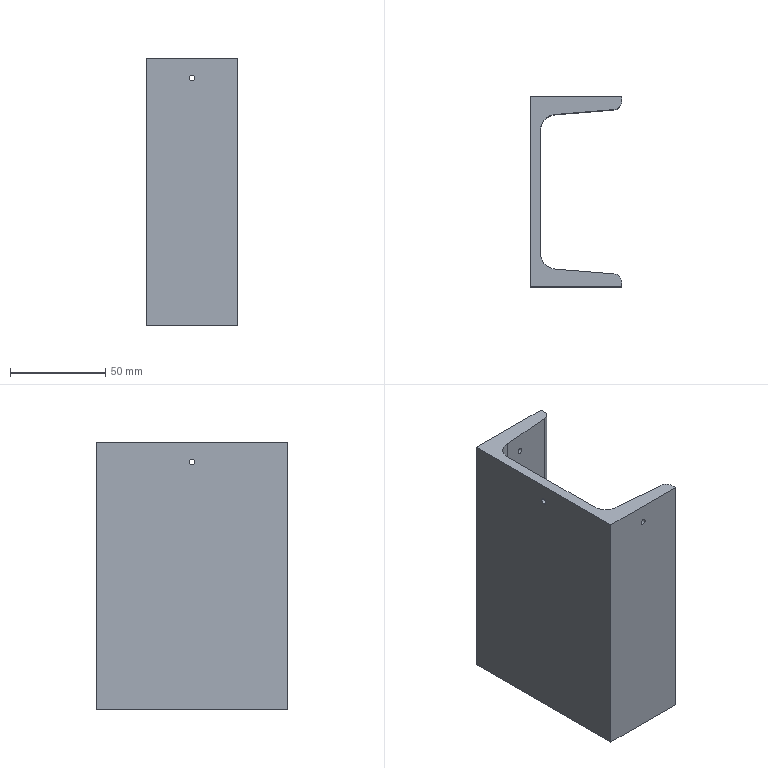Part | STEP file | X77-02212a_10-2 | 1 solid | 20 faces | box 48 x 100 x 140 mm | volume 174699 mm3 | cylinder 10 | plane 10 | commonest cylinder face diameters 3 x6 8.4 x2 17 x2
STEP:
#1=CARTESIAN_POINT('',(25.5,91.708,130.));
#2=VERTEX_POINT('',#1);
#3=CARTESIAN_POINT('',(22.5,91.461,130.));
#4=VERTEX_POINT('',#3);
#5=CARTESIAN_POINT('',(25.5,91.708,130.));
#6=CARTESIAN_POINT('',(25.5,91.708,127.));
#7=CARTESIAN_POINT('',(22.5,91.461,127.));
#8=CARTESIAN_POINT('',(22.5,91.461,130.));
#9=(BOUNDED_CURVE()B_SPLINE_CURVE(3,(#5,#6,#7,#8),.UNSPECIFIED.,.F.,.T.)B_SPLINE_CURVE_WITH_KNOTS((4,4),(0.,3.142),.UNSPECIFIED.)CURVE()GEOMETRIC_REPRESENTATION_ITEM()RATIONAL_B_SPLINE_CURVE((1.,0.3333,0.3333,1.))REPRESENTATION_ITEM(''));
#10=EDGE_CURVE('',#2,#4,#9,.T.);
#11=ORIENTED_EDGE('',*,*,#10,.F.);
#12=CARTESIAN_POINT('',(25.5,100.,130.));
#13=VERTEX_POINT('',#12);
#14=CARTESIAN_POINT('',(25.5,100.,130.));
#15=DIRECTION('',(0.,1.,0.));
#16=VECTOR('',#15,1000.);
#17=LINE('',#14,#16);
#18=EDGE_CURVE('',#2,#13,#17,.T.);
#19=ORIENTED_EDGE('',*,*,#18,.T.);
#20=CARTESIAN_POINT('',(22.5,100.,130.));
#21=VERTEX_POINT('',#20);
#22=CARTESIAN_POINT('',(24.,100.,130.));
#23=DIRECTION('',(0.,1.,0.));
#24=DIRECTION('',(-1.,0.,0.));
#25=AXIS2_PLACEMENT_3D('',#22,#23,#24);
#26=CIRCLE('',#25,1.5);
#27=EDGE_CURVE('',#13,#21,#26,.T.);
#28=ORIENTED_EDGE('',*,*,#27,.T.);
#29=CARTESIAN_POINT('',(22.5,100.,130.));
#30=DIRECTION('',(0.,1.,0.));
#31=VECTOR('',#30,1000.);
#32=LINE('',#29,#31);
#33=EDGE_CURVE('',#4,#21,#32,.T.);
#34=ORIENTED_EDGE('',*,*,#33,.F.);
#35=EDGE_LOOP('',(#11,#19,#28,#34));
#36=FACE_OUTER_BOUND('',#35,.T.);
#37=CARTESIAN_POINT('',(24.,100.,130.));
#38=DIRECTION('',(0.,1.,0.));
#39=DIRECTION('',(-1.,0.,0.));
#40=AXIS2_PLACEMENT_3D('',#37,#38,#39);
#41=CYLINDRICAL_SURFACE('',#40,1.5);
#42=ADVANCED_FACE('',(#36),#41,.F.);
#43=CARTESIAN_POINT('',(25.5,0.,130.));
#44=VERTEX_POINT('',#43);
#45=CARTESIAN_POINT('',(22.5,0.,130.));
#46=VERTEX_POINT('',#45);
#47=CARTESIAN_POINT('',(24.,0.,130.));
#48=DIRECTION('',(0.,1.,0.));
#49=DIRECTION('',(-1.,0.,0.));
#50=AXIS2_PLACEMENT_3D('',#47,#48,#49);
#51=CIRCLE('',#50,1.5);
#52=EDGE_CURVE('',#44,#46,#51,.T.);
#53=ORIENTED_EDGE('',*,*,#52,.F.);
#54=CARTESIAN_POINT('',(25.5,8.292,130.));
#55=VERTEX_POINT('',#54);
#56=CARTESIAN_POINT('',(25.5,100.,130.));
#57=DIRECTION('',(0.,1.,0.));
#58=VECTOR('',#57,1000.);
#59=LINE('',#56,#58);
#60=EDGE_CURVE('',#44,#55,#59,.T.);
#61=ORIENTED_EDGE('',*,*,#60,.T.);
#62=CARTESIAN_POINT('',(22.5,8.539,130.));
#63=VERTEX_POINT('',#62);
#64=CARTESIAN_POINT('',(25.5,8.292,130.));
#65=CARTESIAN_POINT('',(25.5,8.292,127.));
#66=CARTESIAN_POINT('',(22.5,8.539,127.));
#67=CARTESIAN_POINT('',(22.5,8.539,130.));
#68=(BOUNDED_CURVE()B_SPLINE_CURVE(3,(#64,#65,#66,#67),.UNSPECIFIED.,.F.,.F.)B_SPLINE_CURVE_WITH_KNOTS((4,4),(3.142,6.283),.UNSPECIFIED.)CURVE()GEOMETRIC_REPRESENTATION_ITEM()RATIONAL_B_SPLINE_CURVE((1.,0.3333,0.3333,1.))REPRESENTATION_ITEM(''));
#69=EDGE_CURVE('',#55,#63,#68,.T.);
#70=ORIENTED_EDGE('',*,*,#69,.T.);
#71=CARTESIAN_POINT('',(22.5,100.,130.));
#72=DIRECTION('',(0.,1.,0.));
#73=VECTOR('',#72,1000.);
#74=LINE('',#71,#73);
#75=EDGE_CURVE('',#46,#63,#74,.T.);
#76=ORIENTED_EDGE('',*,*,#75,.F.);
#77=EDGE_LOOP('',(#53,#61,#70,#76));
#78=FACE_OUTER_BOUND('',#77,.T.);
#79=CARTESIAN_POINT('',(24.,100.,130.));
#80=DIRECTION('',(0.,1.,0.));
#81=DIRECTION('',(-1.,0.,0.));
#82=AXIS2_PLACEMENT_3D('',#79,#80,#81);
#83=CYLINDRICAL_SURFACE('',#82,1.5);
#84=ADVANCED_FACE('',(#78),#83,.F.);
#85=CARTESIAN_POINT('',(5.3,50.,131.5));
#86=VERTEX_POINT('',#85);
#87=CARTESIAN_POINT('',(5.3,50.,128.5));
#88=VERTEX_POINT('',#87);
#89=CARTESIAN_POINT('',(5.3,50.,130.));
#90=DIRECTION('',(1.,0.,0.));
#91=DIRECTION('',(0.,1.,0.));
#92=AXIS2_PLACEMENT_3D('',#89,#90,#91);
#93=CIRCLE('',#92,1.5);
#94=EDGE_CURVE('',#86,#88,#93,.T.);
#95=ORIENTED_EDGE('',*,*,#94,.T.);
#96=CARTESIAN_POINT('',(0.,50.,128.5));
#97=VERTEX_POINT('',#96);
#98=CARTESIAN_POINT('',(0.,50.,128.5));
#99=DIRECTION('',(-1.,0.,0.));
#100=VECTOR('',#99,1000.);
#101=LINE('',#98,#100);
#102=EDGE_CURVE('',#88,#97,#101,.T.);
#103=ORIENTED_EDGE('',*,*,#102,.T.);
#104=CARTESIAN_POINT('',(0.,50.,131.5));
#105=VERTEX_POINT('',#104);
#106=CARTESIAN_POINT('',(0.,50.,130.));
#107=DIRECTION('',(-1.,0.,0.));
#108=DIRECTION('',(0.,0.,1.));
#109=AXIS2_PLACEMENT_3D('',#106,#107,#108);
#110=CIRCLE('',#109,1.5);
#111=EDGE_CURVE('',#97,#105,#110,.T.);
#112=ORIENTED_EDGE('',*,*,#111,.T.);
#113=CARTESIAN_POINT('',(0.,50.,131.5));
#114=DIRECTION('',(-1.,0.,0.));
#115=VECTOR('',#114,1000.);
#116=LINE('',#113,#115);
#117=EDGE_CURVE('',#86,#105,#116,.T.);
#118=ORIENTED_EDGE('',*,*,#117,.F.);
#119=EDGE_LOOP('',(#95,#103,#112,#118));
#120=FACE_OUTER_BOUND('',#119,.T.);
#121=CARTESIAN_POINT('',(0.,50.,130.));
#122=DIRECTION('',(-1.,0.,0.));
#123=DIRECTION('',(0.,0.,1.));
#124=AXIS2_PLACEMENT_3D('',#121,#122,#123);
#125=CYLINDRICAL_SURFACE('',#124,1.5);
#126=ADVANCED_FACE('',(#120),#125,.F.);
#127=ORIENTED_EDGE('',*,*,#94,.F.);
#128=CARTESIAN_POINT('',(5.3,50.,130.));
#129=DIRECTION('',(1.,0.,0.));
#130=DIRECTION('',(0.,1.,0.));
#131=AXIS2_PLACEMENT_3D('',#128,#129,#130);
#132=CIRCLE('',#131,1.5);
#133=EDGE_CURVE('',#88,#86,#132,.T.);
#134=ORIENTED_EDGE('',*,*,#133,.F.);
#135=EDGE_LOOP('',(#127,#134));
#136=FACE_BOUND('',#135,.T.);
#137=CARTESIAN_POINT('',(5.3,82.245,0.));
#138=VERTEX_POINT('',#137);
#139=CARTESIAN_POINT('',(5.3,17.755,0.));
#140=VERTEX_POINT('',#139);
#141=CARTESIAN_POINT('',(5.3,-36.42,0.));
#142=DIRECTION('',(0.,-1.,0.));
#143=VECTOR('',#142,1000.);
#144=LINE('',#141,#143);
#145=EDGE_CURVE('',#138,#140,#144,.T.);
#146=ORIENTED_EDGE('',*,*,#145,.F.);
#147=CARTESIAN_POINT('',(5.3,82.245,140.));
#148=VERTEX_POINT('',#147);
#149=CARTESIAN_POINT('',(5.3,82.245,140.));
#150=DIRECTION('',(0.,0.,-1.));
#151=VECTOR('',#150,1000.);
#152=LINE('',#149,#151);
#153=EDGE_CURVE('',#148,#138,#152,.T.);
#154=ORIENTED_EDGE('',*,*,#153,.F.);
#155=CARTESIAN_POINT('',(5.3,17.755,140.));
#156=VERTEX_POINT('',#155);
#157=CARTESIAN_POINT('',(5.3,-36.42,140.));
#158=DIRECTION('',(0.,-1.,0.));
#159=VECTOR('',#158,1000.);
#160=LINE('',#157,#159);
#161=EDGE_CURVE('',#148,#156,#160,.T.);
#162=ORIENTED_EDGE('',*,*,#161,.T.);
#163=CARTESIAN_POINT('',(5.3,17.755,140.));
#164=DIRECTION('',(0.,0.,-1.));
#165=VECTOR('',#164,1000.);
#166=LINE('',#163,#165);
#167=EDGE_CURVE('',#156,#140,#166,.T.);
#168=ORIENTED_EDGE('',*,*,#167,.T.);
#169=EDGE_LOOP('',(#146,#154,#162,#168));
#170=FACE_OUTER_BOUND('',#169,.T.);
#171=CARTESIAN_POINT('',(5.3,-36.42,140.));
#172=DIRECTION('',(1.,0.,0.));
#173=DIRECTION('',(0.,0.,-1.));
#174=AXIS2_PLACEMENT_3D('',#171,#172,#173);
#175=PLANE('',#174);
#176=ADVANCED_FACE('',(#136,#170),#175,.T.);
#177=CARTESIAN_POINT('',(13.8,90.745,0.));
#178=VERTEX_POINT('',#177);
#179=CARTESIAN_POINT('',(13.8,82.245,0.));
#180=DIRECTION('',(0.,0.,-1.));
#181=DIRECTION('',(1.,0.,0.));
#182=AXIS2_PLACEMENT_3D('',#179,#180,#181);
#183=CIRCLE('',#182,8.5);
#184=EDGE_CURVE('',#138,#178,#183,.T.);
#185=ORIENTED_EDGE('',*,*,#184,.T.);
#186=CARTESIAN_POINT('',(13.8,90.745,140.));
#187=VERTEX_POINT('',#186);
#188=CARTESIAN_POINT('',(13.8,90.745,140.));
#189=DIRECTION('',(0.,0.,-1.));
#190=VECTOR('',#189,1000.);
#191=LINE('',#188,#190);
#192=EDGE_CURVE('',#187,#178,#191,.T.);
#193=ORIENTED_EDGE('',*,*,#192,.F.);
#194=CARTESIAN_POINT('',(13.8,82.245,140.));
#195=DIRECTION('',(0.,0.,-1.));
#196=DIRECTION('',(1.,0.,0.));
#197=AXIS2_PLACEMENT_3D('',#194,#195,#196);
#198=CIRCLE('',#197,8.5);
#199=EDGE_CURVE('',#148,#187,#198,.T.);
#200=ORIENTED_EDGE('',*,*,#199,.F.);
#201=ORIENTED_EDGE('',*,*,#153,.T.);
#202=EDGE_LOOP('',(#185,#193,#200,#201));
#203=FACE_OUTER_BOUND('',#202,.T.);
#204=CARTESIAN_POINT('',(13.8,82.245,140.));
#205=DIRECTION('',(0.,0.,-1.));
#206=DIRECTION('',(-1.,0.,0.));
#207=AXIS2_PLACEMENT_3D('',#204,#205,#206);
#208=CYLINDRICAL_SURFACE('',#207,8.5);
#209=ADVANCED_FACE('',(#203),#208,.F.);
#210=CARTESIAN_POINT('',(22.5,91.461,130.));
#211=CARTESIAN_POINT('',(22.5,91.461,133.));
#212=CARTESIAN_POINT('',(25.5,91.708,133.));
#213=CARTESIAN_POINT('',(25.5,91.708,130.));
#214=(BOUNDED_CURVE()B_SPLINE_CURVE(3,(#210,#211,#212,#213),.UNSPECIFIED.,.F.,.T.)B_SPLINE_CURVE_WITH_KNOTS((4,4),(3.142,6.283),.UNSPECIFIED.)CURVE()GEOMETRIC_REPRESENTATION_ITEM()RATIONAL_B_SPLINE_CURVE((1.,0.3333,0.3333,1.))REPRESENTATION_ITEM(''));
#215=EDGE_CURVE('',#4,#2,#214,.T.);
#216=ORIENTED_EDGE('',*,*,#215,.T.);
#217=ORIENTED_EDGE('',*,*,#10,.T.);
#218=EDGE_LOOP('',(#216,#217));
#219=FACE_BOUND('',#218,.T.);
#220=CARTESIAN_POINT('',(43.8,93.215,0.));
#221=VERTEX_POINT('',#220);
#222=CARTESIAN_POINT('',(13.532,90.723,0.));
#223=DIRECTION('',(0.9966,0.08206,0.));
#224=VECTOR('',#223,1000.);
#225=LINE('',#222,#224);
#226=EDGE_CURVE('',#178,#221,#225,.T.);
#227=ORIENTED_EDGE('',*,*,#226,.T.);
#228=CARTESIAN_POINT('',(43.8,93.215,140.));
#229=VERTEX_POINT('',#228);
#230=CARTESIAN_POINT('',(43.8,93.215,140.));
#231=DIRECTION('',(0.,0.,-1.));
#232=VECTOR('',#231,1000.);
#233=LINE('',#230,#232);
#234=EDGE_CURVE('',#229,#221,#233,.T.);
#235=ORIENTED_EDGE('',*,*,#234,.F.);
#236=CARTESIAN_POINT('',(13.532,90.723,140.));
#237=DIRECTION('',(0.9966,0.08206,0.));
#238=VECTOR('',#237,1000.);
#239=LINE('',#236,#238);
#240=EDGE_CURVE('',#187,#229,#239,.T.);
#241=ORIENTED_EDGE('',*,*,#240,.F.);
#242=ORIENTED_EDGE('',*,*,#192,.T.);
#243=EDGE_LOOP('',(#227,#235,#241,#242));
#244=FACE_OUTER_BOUND('',#243,.T.);
#245=CARTESIAN_POINT('',(13.532,90.723,140.));
#246=DIRECTION('',(-0.08206,0.9966,0.));
#247=DIRECTION('',(-0.9966,-0.08206,0.));
#248=AXIS2_PLACEMENT_3D('',#245,#246,#247);
#249=PLANE('',#248);
#250=ADVANCED_FACE('',(#219,#244),#249,.F.);
#251=CARTESIAN_POINT('',(48.,97.415,0.));
#252=VERTEX_POINT('',#251);
#253=CARTESIAN_POINT('',(43.8,97.415,0.));
#254=DIRECTION('',(0.,0.,-1.));
#255=DIRECTION('',(1.,0.,0.));
#256=AXIS2_PLACEMENT_3D('',#253,#254,#255);
#257=CIRCLE('',#256,4.2);
#258=EDGE_CURVE('',#252,#221,#257,.T.);
#259=ORIENTED_EDGE('',*,*,#258,.F.);
#260=CARTESIAN_POINT('',(48.,97.415,140.));
#261=VERTEX_POINT('',#260);
#262=CARTESIAN_POINT('',(48.,97.415,140.));
#263=DIRECTION('',(0.,0.,-1.));
#264=VECTOR('',#263,1000.);
#265=LINE('',#262,#264);
#266=EDGE_CURVE('',#261,#252,#265,.T.);
#267=ORIENTED_EDGE('',*,*,#266,.F.);
#268=CARTESIAN_POINT('',(43.8,97.415,140.));
#269=DIRECTION('',(0.,0.,-1.));
#270=DIRECTION('',(1.,0.,0.));
#271=AXIS2_PLACEMENT_3D('',#268,#269,#270);
#272=CIRCLE('',#271,4.2);
#273=EDGE_CURVE('',#261,#229,#272,.T.);
#274=ORIENTED_EDGE('',*,*,#273,.T.);
#275=ORIENTED_EDGE('',*,*,#234,.T.);
#276=EDGE_LOOP('',(#259,#267,#274,#275));
#277=FACE_OUTER_BOUND('',#276,.T.);
#278=CARTESIAN_POINT('',(43.8,97.415,140.));
#279=DIRECTION('',(0.,0.,-1.));
#280=DIRECTION('',(-1.,0.,0.));
#281=AXIS2_PLACEMENT_3D('',#278,#279,#280);
#282=CYLINDRICAL_SURFACE('',#281,4.2);
#283=ADVANCED_FACE('',(#277),#282,.T.);
#284=CARTESIAN_POINT('',(48.,100.,0.));
#285=VERTEX_POINT('',#284);
#286=CARTESIAN_POINT('',(48.,-36.42,0.));
#287=DIRECTION('',(0.,-1.,0.));
#288=VECTOR('',#287,1000.);
#289=LINE('',#286,#288);
#290=EDGE_CURVE('',#285,#252,#289,.T.);
#291=ORIENTED_EDGE('',*,*,#290,.F.);
#292=CARTESIAN_POINT('',(48.,100.,140.));
#293=VERTEX_POINT('',#292);
#294=CARTESIAN_POINT('',(48.,100.,140.));
#295=DIRECTION('',(0.,0.,-1.));
#296=VECTOR('',#295,1000.);
#297=LINE('',#294,#296);
#298=EDGE_CURVE('',#293,#285,#297,.T.);
#299=ORIENTED_EDGE('',*,*,#298,.F.);
#300=CARTESIAN_POINT('',(48.,-36.42,140.));
#301=DIRECTION('',(0.,-1.,0.));
#302=VECTOR('',#301,1000.);
#303=LINE('',#300,#302);
#304=EDGE_CURVE('',#293,#261,#303,.T.);
#305=ORIENTED_EDGE('',*,*,#304,.T.);
#306=ORIENTED_EDGE('',*,*,#266,.T.);
#307=EDGE_LOOP('',(#291,#299,#305,#306));
#308=FACE_OUTER_BOUND('',#307,.T.);
#309=CARTESIAN_POINT('',(48.,-36.42,140.));
#310=DIRECTION('',(1.,0.,0.));
#311=DIRECTION('',(0.,0.,-1.));
#312=AXIS2_PLACEMENT_3D('',#309,#310,#311);
#313=PLANE('',#312);
#314=ADVANCED_FACE('',(#308),#313,.T.);
#315=CARTESIAN_POINT('',(24.,100.,130.));
#316=DIRECTION('',(0.,1.,0.));
#317=DIRECTION('',(-1.,0.,0.));
#318=AXIS2_PLACEMENT_3D('',#315,#316,#317);
#319=CIRCLE('',#318,1.5);
#320=EDGE_CURVE('',#21,#13,#319,.T.);
#321=ORIENTED_EDGE('',*,*,#320,.F.);
#322=ORIENTED_EDGE('',*,*,#27,.F.);
#323=EDGE_LOOP('',(#321,#322));
#324=FACE_BOUND('',#323,.T.);
#325=CARTESIAN_POINT('',(0.,100.,0.));
#326=VERTEX_POINT('',#325);
#327=CARTESIAN_POINT('',(24.,100.,0.));
#328=DIRECTION('',(1.,0.,0.));
#329=VECTOR('',#328,1000.);
#330=LINE('',#327,#329);
#331=EDGE_CURVE('',#326,#285,#330,.T.);
#332=ORIENTED_EDGE('',*,*,#331,.F.);
#333=CARTESIAN_POINT('',(0.,100.,140.));
#334=VERTEX_POINT('',#333);
#335=CARTESIAN_POINT('',(0.,100.,140.));
#336=DIRECTION('',(0.,0.,-1.));
#337=VECTOR('',#336,1000.);
#338=LINE('',#335,#337);
#339=EDGE_CURVE('',#334,#326,#338,.T.);
#340=ORIENTED_EDGE('',*,*,#339,.F.);
#341=CARTESIAN_POINT('',(24.,100.,140.));
#342=DIRECTION('',(1.,0.,0.));
#343=VECTOR('',#342,1000.);
#344=LINE('',#341,#343);
#345=EDGE_CURVE('',#334,#293,#344,.T.);
#346=ORIENTED_EDGE('',*,*,#345,.T.);
#347=ORIENTED_EDGE('',*,*,#298,.T.);
#348=EDGE_LOOP('',(#332,#340,#346,#347));
#349=FACE_OUTER_BOUND('',#348,.T.);
#350=CARTESIAN_POINT('',(24.,100.,140.));
#351=DIRECTION('',(0.,1.,0.));
#352=DIRECTION('',(0.,0.,1.));
#353=AXIS2_PLACEMENT_3D('',#350,#351,#352);
#354=PLANE('',#353);
#355=ADVANCED_FACE('',(#324,#349),#354,.T.);
#356=CARTESIAN_POINT('',(0.,50.,130.));
#357=DIRECTION('',(-1.,0.,0.));
#358=DIRECTION('',(0.,0.,1.));
#359=AXIS2_PLACEMENT_3D('',#356,#357,#358);
#360=CIRCLE('',#359,1.5);
#361=EDGE_CURVE('',#105,#97,#360,.T.);
#362=ORIENTED_EDGE('',*,*,#361,.F.);
#363=ORIENTED_EDGE('',*,*,#111,.F.);
#364=EDGE_LOOP('',(#362,#363));
#365=FACE_BOUND('',#364,.T.);
#366=CARTESIAN_POINT('',(0.,0.,0.));
#367=VERTEX_POINT('',#366);
#368=CARTESIAN_POINT('',(0.,-36.42,0.));
#369=DIRECTION('',(0.,1.,0.));
#370=VECTOR('',#369,1000.);
#371=LINE('',#368,#370);
#372=EDGE_CURVE('',#367,#326,#371,.T.);
#373=ORIENTED_EDGE('',*,*,#372,.F.);
#374=CARTESIAN_POINT('',(0.,0.,140.));
#375=VERTEX_POINT('',#374);
#376=CARTESIAN_POINT('',(0.,0.,140.));
#377=DIRECTION('',(0.,0.,-1.));
#378=VECTOR('',#377,1000.);
#379=LINE('',#376,#378);
#380=EDGE_CURVE('',#375,#367,#379,.T.);
#381=ORIENTED_EDGE('',*,*,#380,.F.);
#382=CARTESIAN_POINT('',(0.,-36.42,140.));
#383=DIRECTION('',(0.,1.,0.));
#384=VECTOR('',#383,1000.);
#385=LINE('',#382,#384);
#386=EDGE_CURVE('',#375,#334,#385,.T.);
#387=ORIENTED_EDGE('',*,*,#386,.T.);
#388=ORIENTED_EDGE('',*,*,#339,.T.);
#389=EDGE_LOOP('',(#373,#381,#387,#388));
#390=FACE_OUTER_BOUND('',#389,.T.);
#391=CARTESIAN_POINT('',(0.,-36.42,140.));
#392=DIRECTION('',(-1.,0.,0.));
#393=DIRECTION('',(0.,0.,1.));
#394=AXIS2_PLACEMENT_3D('',#391,#392,#393);
#395=PLANE('',#394);
#396=ADVANCED_FACE('',(#365,#390),#395,.T.);
#397=CARTESIAN_POINT('',(24.,0.,130.));
#398=DIRECTION('',(0.,1.,0.));
#399=DIRECTION('',(-1.,0.,0.));
#400=AXIS2_PLACEMENT_3D('',#397,#398,#399);
#401=CIRCLE('',#400,1.5);
#402=EDGE_CURVE('',#46,#44,#401,.T.);
#403=ORIENTED_EDGE('',*,*,#402,.T.);
#404=ORIENTED_EDGE('',*,*,#52,.T.);
#405=EDGE_LOOP('',(#403,#404));
#406=FACE_BOUND('',#405,.T.);
#407=CARTESIAN_POINT('',(48.,0.,0.));
#408=VERTEX_POINT('',#407);
#409=CARTESIAN_POINT('',(24.,0.,0.));
#410=DIRECTION('',(1.,0.,0.));
#411=VECTOR('',#410,1000.);
#412=LINE('',#409,#411);
#413=EDGE_CURVE('',#367,#408,#412,.T.);
#414=ORIENTED_EDGE('',*,*,#413,.T.);
#415=CARTESIAN_POINT('',(48.,0.,140.));
#416=VERTEX_POINT('',#415);
#417=CARTESIAN_POINT('',(48.,0.,140.));
#418=DIRECTION('',(0.,0.,-1.));
#419=VECTOR('',#418,1000.);
#420=LINE('',#417,#419);
#421=EDGE_CURVE('',#416,#408,#420,.T.);
#422=ORIENTED_EDGE('',*,*,#421,.F.);
#423=CARTESIAN_POINT('',(24.,0.,140.));
#424=DIRECTION('',(1.,0.,0.));
#425=VECTOR('',#424,1000.);
#426=LINE('',#423,#425);
#427=EDGE_CURVE('',#375,#416,#426,.T.);
#428=ORIENTED_EDGE('',*,*,#427,.F.);
#429=ORIENTED_EDGE('',*,*,#380,.T.);
#430=EDGE_LOOP('',(#414,#422,#428,#429));
#431=FACE_OUTER_BOUND('',#430,.T.);
#432=CARTESIAN_POINT('',(24.,0.,140.));
#433=DIRECTION('',(0.,1.,0.));
#434=DIRECTION('',(0.,0.,1.));
#435=AXIS2_PLACEMENT_3D('',#432,#433,#434);
#436=PLANE('',#435);
#437=ADVANCED_FACE('',(#406,#431),#436,.F.);
#438=CARTESIAN_POINT('',(48.,2.585,0.));
#439=VERTEX_POINT('',#438);
#440=CARTESIAN_POINT('',(48.,-36.42,0.));
#441=DIRECTION('',(0.,1.,0.));
#442=VECTOR('',#441,1000.);
#443=LINE('',#440,#442);
#444=EDGE_CURVE('',#408,#439,#443,.T.);
#445=ORIENTED_EDGE('',*,*,#444,.T.);
#446=CARTESIAN_POINT('',(48.,2.585,140.));
#447=VERTEX_POINT('',#446);
#448=CARTESIAN_POINT('',(48.,2.585,140.));
#449=DIRECTION('',(0.,0.,-1.));
#450=VECTOR('',#449,1000.);
#451=LINE('',#448,#450);
#452=EDGE_CURVE('',#447,#439,#451,.T.);
#453=ORIENTED_EDGE('',*,*,#452,.F.);
#454=CARTESIAN_POINT('',(48.,-36.42,140.));
#455=DIRECTION('',(0.,1.,0.));
#456=VECTOR('',#455,1000.);
#457=LINE('',#454,#456);
#458=EDGE_CURVE('',#416,#447,#457,.T.);
#459=ORIENTED_EDGE('',*,*,#458,.F.);
#460=ORIENTED_EDGE('',*,*,#421,.T.);
#461=EDGE_LOOP('',(#445,#453,#459,#460));
#462=FACE_OUTER_BOUND('',#461,.T.);
#463=CARTESIAN_POINT('',(48.,-36.42,140.));
#464=DIRECTION('',(-1.,0.,0.));
#465=DIRECTION('',(0.,0.,1.));
#466=AXIS2_PLACEMENT_3D('',#463,#464,#465);
#467=PLANE('',#466);
#468=ADVANCED_FACE('',(#462),#467,.F.);
#469=CARTESIAN_POINT('',(43.8,6.785,0.));
#470=VERTEX_POINT('',#469);
#471=CARTESIAN_POINT('',(43.8,2.585,0.));
#472=DIRECTION('',(0.,0.,1.));
#473=DIRECTION('',(1.,0.,0.));
#474=AXIS2_PLACEMENT_3D('',#471,#472,#473);
#475=CIRCLE('',#474,4.2);
#476=EDGE_CURVE('',#439,#470,#475,.T.);
#477=ORIENTED_EDGE('',*,*,#476,.T.);
#478=CARTESIAN_POINT('',(43.8,6.785,140.));
#479=VERTEX_POINT('',#478);
#480=CARTESIAN_POINT('',(43.8,6.785,140.));
#481=DIRECTION('',(0.,0.,-1.));
#482=VECTOR('',#481,1000.);
#483=LINE('',#480,#482);
#484=EDGE_CURVE('',#479,#470,#483,.T.);
#485=ORIENTED_EDGE('',*,*,#484,.F.);
#486=CARTESIAN_POINT('',(43.8,2.585,140.));
#487=DIRECTION('',(0.,0.,1.));
#488=DIRECTION('',(1.,0.,0.));
#489=AXIS2_PLACEMENT_3D('',#486,#487,#488);
#490=CIRCLE('',#489,4.2);
#491=EDGE_CURVE('',#447,#479,#490,.T.);
#492=ORIENTED_EDGE('',*,*,#491,.F.);
#493=ORIENTED_EDGE('',*,*,#452,.T.);
#494=EDGE_LOOP('',(#477,#485,#492,#493));
#495=FACE_OUTER_BOUND('',#494,.T.);
#496=CARTESIAN_POINT('',(43.8,2.585,140.));
#497=DIRECTION('',(0.,0.,-1.));
#498=DIRECTION('',(-1.,0.,0.));
#499=AXIS2_PLACEMENT_3D('',#496,#497,#498);
#500=CYLINDRICAL_SURFACE('',#499,4.2);
#501=ADVANCED_FACE('',(#495),#500,.T.);
#502=CARTESIAN_POINT('',(22.5,8.539,130.));
#503=CARTESIAN_POINT('',(22.5,8.539,133.));
#504=CARTESIAN_POINT('',(25.5,8.292,133.));
#505=CARTESIAN_POINT('',(25.5,8.292,130.));
#506=(BOUNDED_CURVE()B_SPLINE_CURVE(3,(#502,#503,#504,#505),.UNSPECIFIED.,.F.,.F.)B_SPLINE_CURVE_WITH_KNOTS((4,4),(0.,3.142),.UNSPECIFIED.)CURVE()GEOMETRIC_REPRESENTATION_ITEM()RATIONAL_B_SPLINE_CURVE((1.,0.3333,0.3333,1.))REPRESENTATION_ITEM(''));
#507=EDGE_CURVE('',#63,#55,#506,.T.);
#508=ORIENTED_EDGE('',*,*,#507,.F.);
#509=ORIENTED_EDGE('',*,*,#69,.F.);
#510=EDGE_LOOP('',(#508,#509));
#511=FACE_BOUND('',#510,.T.);
#512=CARTESIAN_POINT('',(13.8,9.255,0.));
#513=VERTEX_POINT('',#512);
#514=CARTESIAN_POINT('',(27.667,8.113,0.));
#515=DIRECTION('',(0.9966,-0.08206,0.));
#516=VECTOR('',#515,1000.);
#517=LINE('',#514,#516);
#518=EDGE_CURVE('',#513,#470,#517,.T.);
#519=ORIENTED_EDGE('',*,*,#518,.F.);
#520=CARTESIAN_POINT('',(13.8,9.255,140.));
#521=VERTEX_POINT('',#520);
#522=CARTESIAN_POINT('',(13.8,9.255,140.));
#523=DIRECTION('',(0.,0.,-1.));
#524=VECTOR('',#523,1000.);
#525=LINE('',#522,#524);
#526=EDGE_CURVE('',#521,#513,#525,.T.);
#527=ORIENTED_EDGE('',*,*,#526,.F.);
#528=CARTESIAN_POINT('',(27.667,8.113,140.));
#529=DIRECTION('',(0.9966,-0.08206,0.));
#530=VECTOR('',#529,1000.);
#531=LINE('',#528,#530);
#532=EDGE_CURVE('',#521,#479,#531,.T.);
#533=ORIENTED_EDGE('',*,*,#532,.T.);
#534=ORIENTED_EDGE('',*,*,#484,.T.);
#535=EDGE_LOOP('',(#519,#527,#533,#534));
#536=FACE_OUTER_BOUND('',#535,.T.);
#537=CARTESIAN_POINT('',(27.667,8.113,140.));
#538=DIRECTION('',(0.08206,0.9966,0.));
#539=DIRECTION('',(-0.9966,0.08206,0.));
#540=AXIS2_PLACEMENT_3D('',#537,#538,#539);
#541=PLANE('',#540);
#542=ADVANCED_FACE('',(#511,#536),#541,.T.);
#543=CARTESIAN_POINT('',(13.8,17.755,0.));
#544=DIRECTION('',(0.,0.,1.));
#545=DIRECTION('',(1.,0.,0.));
#546=AXIS2_PLACEMENT_3D('',#543,#544,#545);
#547=CIRCLE('',#546,8.5);
#548=EDGE_CURVE('',#140,#513,#547,.T.);
#549=ORIENTED_EDGE('',*,*,#548,.F.);
#550=ORIENTED_EDGE('',*,*,#167,.F.);
#551=CARTESIAN_POINT('',(13.8,17.755,140.));
#552=DIRECTION('',(0.,0.,1.));
#553=DIRECTION('',(1.,0.,0.));
#554=AXIS2_PLACEMENT_3D('',#551,#552,#553);
#555=CIRCLE('',#554,8.5);
#556=EDGE_CURVE('',#156,#521,#555,.T.);
#557=ORIENTED_EDGE('',*,*,#556,.T.);
#558=ORIENTED_EDGE('',*,*,#526,.T.);
#559=EDGE_LOOP('',(#549,#550,#557,#558));
#560=FACE_OUTER_BOUND('',#559,.T.);
#561=CARTESIAN_POINT('',(13.8,17.755,140.));
#562=DIRECTION('',(0.,0.,-1.));
#563=DIRECTION('',(-1.,0.,0.));
#564=AXIS2_PLACEMENT_3D('',#561,#562,#563);
#565=CYLINDRICAL_SURFACE('',#564,8.5);
#566=ADVANCED_FACE('',(#560),#565,.F.);
#567=ORIENTED_EDGE('',*,*,#491,.T.);
#568=ORIENTED_EDGE('',*,*,#532,.F.);
#569=ORIENTED_EDGE('',*,*,#556,.F.);
#570=ORIENTED_EDGE('',*,*,#161,.F.);
#571=ORIENTED_EDGE('',*,*,#199,.T.);
#572=ORIENTED_EDGE('',*,*,#240,.T.);
#573=ORIENTED_EDGE('',*,*,#273,.F.);
#574=ORIENTED_EDGE('',*,*,#304,.F.);
#575=ORIENTED_EDGE('',*,*,#345,.F.);
#576=ORIENTED_EDGE('',*,*,#386,.F.);
#577=ORIENTED_EDGE('',*,*,#427,.T.);
#578=ORIENTED_EDGE('',*,*,#458,.T.);
#579=EDGE_LOOP('',(#567,#568,#569,#570,#571,#572,#573,#574,#575,#576,#577,#578));
#580=FACE_OUTER_BOUND('',#579,.T.);
#581=CARTESIAN_POINT('',(24.,-36.42,140.));
#582=DIRECTION('',(0.,0.,1.));
#583=DIRECTION('',(1.,0.,0.));
#584=AXIS2_PLACEMENT_3D('',#581,#582,#583);
#585=PLANE('',#584);
#586=ADVANCED_FACE('',(#580),#585,.T.);
#587=ORIENTED_EDGE('',*,*,#145,.T.);
#588=ORIENTED_EDGE('',*,*,#548,.T.);
#589=ORIENTED_EDGE('',*,*,#518,.T.);
#590=ORIENTED_EDGE('',*,*,#476,.F.);
#591=ORIENTED_EDGE('',*,*,#444,.F.);
#592=ORIENTED_EDGE('',*,*,#413,.F.);
#593=ORIENTED_EDGE('',*,*,#372,.T.);
#594=ORIENTED_EDGE('',*,*,#331,.T.);
#595=ORIENTED_EDGE('',*,*,#290,.T.);
#596=ORIENTED_EDGE('',*,*,#258,.T.);
#597=ORIENTED_EDGE('',*,*,#226,.F.);
#598=ORIENTED_EDGE('',*,*,#184,.F.);
#599=EDGE_LOOP('',(#587,#588,#589,#590,#591,#592,#593,#594,#595,#596,#597,#598));
#600=FACE_OUTER_BOUND('',#599,.T.);
#601=CARTESIAN_POINT('',(24.,-36.42,0.));
#602=DIRECTION('',(0.,0.,1.));
#603=DIRECTION('',(1.,0.,0.));
#604=AXIS2_PLACEMENT_3D('',#601,#602,#603);
#605=PLANE('',#604);
#606=ADVANCED_FACE('',(#600),#605,.F.);
#607=ORIENTED_EDGE('',*,*,#102,.F.);
#608=ORIENTED_EDGE('',*,*,#133,.T.);
#609=ORIENTED_EDGE('',*,*,#117,.T.);
#610=ORIENTED_EDGE('',*,*,#361,.T.);
#611=EDGE_LOOP('',(#607,#608,#609,#610));
#612=FACE_OUTER_BOUND('',#611,.T.);
#613=CARTESIAN_POINT('',(0.,50.,130.));
#614=DIRECTION('',(-1.,0.,0.));
#615=DIRECTION('',(0.,0.,1.));
#616=AXIS2_PLACEMENT_3D('',#613,#614,#615);
#617=CYLINDRICAL_SURFACE('',#616,1.5);
#618=ADVANCED_FACE('',(#612),#617,.F.);
#619=ORIENTED_EDGE('',*,*,#60,.F.);
#620=ORIENTED_EDGE('',*,*,#402,.F.);
#621=ORIENTED_EDGE('',*,*,#75,.T.);
#622=ORIENTED_EDGE('',*,*,#507,.T.);
#623=EDGE_LOOP('',(#619,#620,#621,#622));
#624=FACE_OUTER_BOUND('',#623,.T.);
#625=CARTESIAN_POINT('',(24.,100.,130.));
#626=DIRECTION('',(0.,1.,0.));
#627=DIRECTION('',(-1.,0.,0.));
#628=AXIS2_PLACEMENT_3D('',#625,#626,#627);
#629=CYLINDRICAL_SURFACE('',#628,1.5);
#630=ADVANCED_FACE('',(#624),#629,.F.);
#631=ORIENTED_EDGE('',*,*,#18,.F.);
#632=ORIENTED_EDGE('',*,*,#215,.F.);
#633=ORIENTED_EDGE('',*,*,#33,.T.);
#634=ORIENTED_EDGE('',*,*,#320,.T.);
#635=EDGE_LOOP('',(#631,#632,#633,#634));
#636=FACE_OUTER_BOUND('',#635,.T.);
#637=CARTESIAN_POINT('',(24.,100.,130.));
#638=DIRECTION('',(0.,1.,0.));
#639=DIRECTION('',(-1.,0.,0.));
#640=AXIS2_PLACEMENT_3D('',#637,#638,#639);
#641=CYLINDRICAL_SURFACE('',#640,1.5);
#642=ADVANCED_FACE('',(#636),#641,.F.);
#643=CLOSED_SHELL('',(#42,#84,#126,#176,#209,#250,#283,#314,#355,#396,#437,#468,#501,#542,#566,#586,#606,#618,#630,#642));
#644=MANIFOLD_SOLID_BREP('',#643);
#645=CARTESIAN_POINT('',(0.,0.,0.));
#646=DIRECTION('',(0.,0.,1.));
#647=DIRECTION('',(1.,0.,0.));
#648=AXIS2_PLACEMENT_3D('',#645,#646,#647);
#649=(LENGTH_UNIT()NAMED_UNIT(*)SI_UNIT(.MILLI.,.METRE.));
#650=UNCERTAINTY_MEASURE_WITH_UNIT(LENGTH_MEASURE(0.00001),#649,'','');
#651=(NAMED_UNIT(*)PLANE_ANGLE_UNIT()SI_UNIT($,.RADIAN.));
#652=(NAMED_UNIT(*)SI_UNIT($,.STERADIAN.)SOLID_ANGLE_UNIT());
#653=(GEOMETRIC_REPRESENTATION_CONTEXT(3)GLOBAL_UNCERTAINTY_ASSIGNED_CONTEXT((#650))GLOBAL_UNIT_ASSIGNED_CONTEXT((#649,#651,#652))REPRESENTATION_CONTEXT('',''));
#654=ADVANCED_BREP_SHAPE_REPRESENTATION('',(#644,#648),#653);